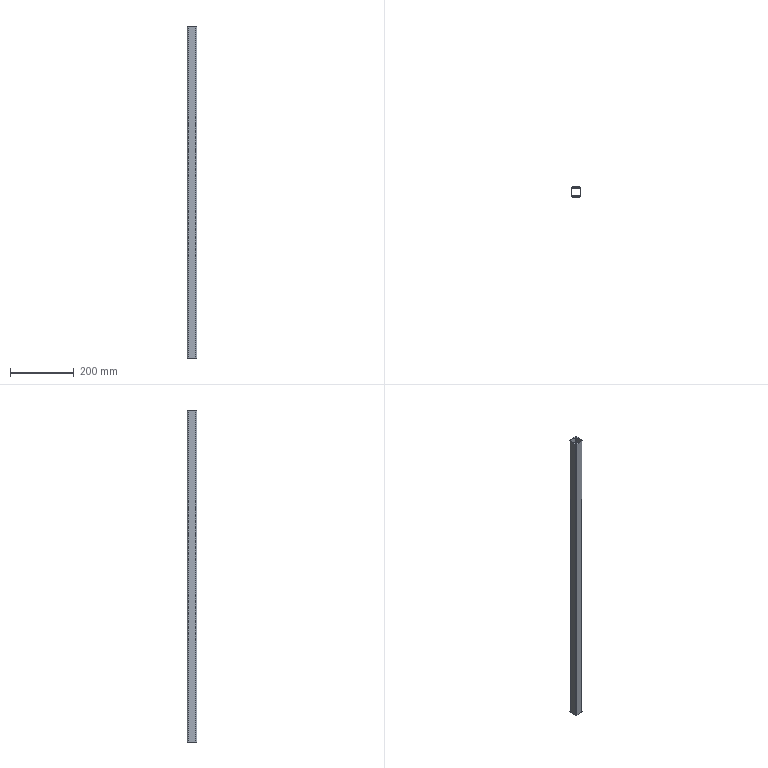Part | SolidWorks | features Attribute 1, ExtruThin 1 | 1 solid | 18 faces | box 30 x 30 x 1038 mm | volume 221734 mm3 | plane 10 | cylinder 8 | commonest cylinder face diameters 4 x4 8 x4
STEP:
#1=CARTESIAN_POINT('',(15.,11.,518.8));
#2=VERTEX_POINT('',#1);
#3=CARTESIAN_POINT('',(11.,15.,518.8));
#4=VERTEX_POINT('',#3);
#5=CARTESIAN_POINT('',(11.,11.,518.8));
#6=DIRECTION('',(0.,0.,1.));
#7=DIRECTION('',(1.,0.,0.));
#8=AXIS2_PLACEMENT_3D('',#5,#6,#7);
#9=CIRCLE('',#8,4.);
#10=EDGE_CURVE('',#2,#4,#9,.T.);
#11=ORIENTED_EDGE('',*,*,#10,.T.);
#12=CARTESIAN_POINT('',(-11.,15.,518.8));
#13=VERTEX_POINT('',#12);
#14=CARTESIAN_POINT('',(11.,15.,518.8));
#15=DIRECTION('',(-1.,0.,0.));
#16=VECTOR('',#15,1000.);
#17=LINE('',#14,#16);
#18=EDGE_CURVE('',#4,#13,#17,.T.);
#19=ORIENTED_EDGE('',*,*,#18,.T.);
#20=CARTESIAN_POINT('',(-15.,11.,518.8));
#21=VERTEX_POINT('',#20);
#22=CARTESIAN_POINT('',(-11.,11.,518.8));
#23=DIRECTION('',(0.,0.,1.));
#24=DIRECTION('',(1.,0.,0.));
#25=AXIS2_PLACEMENT_3D('',#22,#23,#24);
#26=CIRCLE('',#25,4.);
#27=EDGE_CURVE('',#13,#21,#26,.T.);
#28=ORIENTED_EDGE('',*,*,#27,.T.);
#29=CARTESIAN_POINT('',(-15.,-11.,518.8));
#30=VERTEX_POINT('',#29);
#31=CARTESIAN_POINT('',(-15.,-11.,518.8));
#32=DIRECTION('',(0.,1.,0.));
#33=VECTOR('',#32,1000.);
#34=LINE('',#31,#33);
#35=EDGE_CURVE('',#30,#21,#34,.T.);
#36=ORIENTED_EDGE('',*,*,#35,.F.);
#37=CARTESIAN_POINT('',(-11.,-15.,518.8));
#38=VERTEX_POINT('',#37);
#39=CARTESIAN_POINT('',(-11.,-11.,518.8));
#40=DIRECTION('',(0.,0.,1.));
#41=DIRECTION('',(1.,0.,0.));
#42=AXIS2_PLACEMENT_3D('',#39,#40,#41);
#43=CIRCLE('',#42,4.);
#44=EDGE_CURVE('',#30,#38,#43,.T.);
#45=ORIENTED_EDGE('',*,*,#44,.T.);
#46=CARTESIAN_POINT('',(11.,-15.,518.8));
#47=VERTEX_POINT('',#46);
#48=CARTESIAN_POINT('',(-11.,-15.,518.8));
#49=DIRECTION('',(1.,0.,0.));
#50=VECTOR('',#49,1000.);
#51=LINE('',#48,#50);
#52=EDGE_CURVE('',#38,#47,#51,.T.);
#53=ORIENTED_EDGE('',*,*,#52,.T.);
#54=CARTESIAN_POINT('',(15.,-11.,518.8));
#55=VERTEX_POINT('',#54);
#56=CARTESIAN_POINT('',(11.,-11.,518.8));
#57=DIRECTION('',(0.,0.,1.));
#58=DIRECTION('',(1.,0.,0.));
#59=AXIS2_PLACEMENT_3D('',#56,#57,#58);
#60=CIRCLE('',#59,4.);
#61=EDGE_CURVE('',#47,#55,#60,.T.);
#62=ORIENTED_EDGE('',*,*,#61,.T.);
#63=CARTESIAN_POINT('',(15.,11.,518.8));
#64=DIRECTION('',(0.,-1.,0.));
#65=VECTOR('',#64,1000.);
#66=LINE('',#63,#65);
#67=EDGE_CURVE('',#2,#55,#66,.T.);
#68=ORIENTED_EDGE('',*,*,#67,.F.);
#69=EDGE_LOOP('',(#11,#19,#28,#36,#45,#53,#62,#68));
#70=FACE_OUTER_BOUND('',#69,.T.);
#71=CARTESIAN_POINT('',(11.,13.,518.8));
#72=VERTEX_POINT('',#71);
#73=CARTESIAN_POINT('',(-11.,13.,518.8));
#74=VERTEX_POINT('',#73);
#75=CARTESIAN_POINT('',(11.,13.,518.8));
#76=DIRECTION('',(-1.,0.,0.));
#77=VECTOR('',#76,1000.);
#78=LINE('',#75,#77);
#79=EDGE_CURVE('',#72,#74,#78,.T.);
#80=ORIENTED_EDGE('',*,*,#79,.F.);
#81=CARTESIAN_POINT('',(13.,11.,518.8));
#82=VERTEX_POINT('',#81);
#83=CARTESIAN_POINT('',(11.,11.,518.8));
#84=DIRECTION('',(0.,0.,1.));
#85=DIRECTION('',(1.,0.,0.));
#86=AXIS2_PLACEMENT_3D('',#83,#84,#85);
#87=CIRCLE('',#86,2.);
#88=EDGE_CURVE('',#82,#72,#87,.T.);
#89=ORIENTED_EDGE('',*,*,#88,.F.);
#90=CARTESIAN_POINT('',(13.,-11.,518.8));
#91=VERTEX_POINT('',#90);
#92=CARTESIAN_POINT('',(13.,11.,518.8));
#93=DIRECTION('',(0.,-1.,0.));
#94=VECTOR('',#93,1000.);
#95=LINE('',#92,#94);
#96=EDGE_CURVE('',#82,#91,#95,.T.);
#97=ORIENTED_EDGE('',*,*,#96,.T.);
#98=CARTESIAN_POINT('',(11.,-13.,518.8));
#99=VERTEX_POINT('',#98);
#100=CARTESIAN_POINT('',(11.,-11.,518.8));
#101=DIRECTION('',(0.,0.,1.));
#102=DIRECTION('',(1.,0.,0.));
#103=AXIS2_PLACEMENT_3D('',#100,#101,#102);
#104=CIRCLE('',#103,2.);
#105=EDGE_CURVE('',#99,#91,#104,.T.);
#106=ORIENTED_EDGE('',*,*,#105,.F.);
#107=CARTESIAN_POINT('',(-11.,-13.,518.8));
#108=VERTEX_POINT('',#107);
#109=CARTESIAN_POINT('',(-11.,-13.,518.8));
#110=DIRECTION('',(1.,0.,0.));
#111=VECTOR('',#110,1000.);
#112=LINE('',#109,#111);
#113=EDGE_CURVE('',#108,#99,#112,.T.);
#114=ORIENTED_EDGE('',*,*,#113,.F.);
#115=CARTESIAN_POINT('',(-13.,-11.,518.8));
#116=VERTEX_POINT('',#115);
#117=CARTESIAN_POINT('',(-11.,-11.,518.8));
#118=DIRECTION('',(0.,0.,1.));
#119=DIRECTION('',(1.,0.,0.));
#120=AXIS2_PLACEMENT_3D('',#117,#118,#119);
#121=CIRCLE('',#120,2.);
#122=EDGE_CURVE('',#116,#108,#121,.T.);
#123=ORIENTED_EDGE('',*,*,#122,.F.);
#124=CARTESIAN_POINT('',(-13.,11.,518.8));
#125=VERTEX_POINT('',#124);
#126=CARTESIAN_POINT('',(-13.,-11.,518.8));
#127=DIRECTION('',(0.,1.,0.));
#128=VECTOR('',#127,1000.);
#129=LINE('',#126,#128);
#130=EDGE_CURVE('',#116,#125,#129,.T.);
#131=ORIENTED_EDGE('',*,*,#130,.T.);
#132=CARTESIAN_POINT('',(-11.,11.,518.8));
#133=DIRECTION('',(0.,0.,1.));
#134=DIRECTION('',(1.,0.,0.));
#135=AXIS2_PLACEMENT_3D('',#132,#133,#134);
#136=CIRCLE('',#135,2.);
#137=EDGE_CURVE('',#74,#125,#136,.T.);
#138=ORIENTED_EDGE('',*,*,#137,.F.);
#139=EDGE_LOOP('',(#80,#89,#97,#106,#114,#123,#131,#138));
#140=FACE_BOUND('',#139,.T.);
#141=CARTESIAN_POINT('',(11.,11.,518.8));
#142=DIRECTION('',(0.,0.,1.));
#143=DIRECTION('',(1.,0.,0.));
#144=AXIS2_PLACEMENT_3D('',#141,#142,#143);
#145=PLANE('',#144);
#146=ADVANCED_FACE('',(#70,#140),#145,.T.);
#147=CARTESIAN_POINT('',(15.,11.,-518.8));
#148=VERTEX_POINT('',#147);
#149=CARTESIAN_POINT('',(11.,15.,-518.8));
#150=VERTEX_POINT('',#149);
#151=CARTESIAN_POINT('',(11.,11.,-518.8));
#152=DIRECTION('',(0.,0.,1.));
#153=DIRECTION('',(1.,0.,0.));
#154=AXIS2_PLACEMENT_3D('',#151,#152,#153);
#155=CIRCLE('',#154,4.);
#156=EDGE_CURVE('',#148,#150,#155,.T.);
#157=ORIENTED_EDGE('',*,*,#156,.F.);
#158=CARTESIAN_POINT('',(15.,-11.,-518.8));
#159=VERTEX_POINT('',#158);
#160=CARTESIAN_POINT('',(15.,11.,-518.8));
#161=DIRECTION('',(0.,-1.,0.));
#162=VECTOR('',#161,1000.);
#163=LINE('',#160,#162);
#164=EDGE_CURVE('',#148,#159,#163,.T.);
#165=ORIENTED_EDGE('',*,*,#164,.T.);
#166=CARTESIAN_POINT('',(11.,-15.,-518.8));
#167=VERTEX_POINT('',#166);
#168=CARTESIAN_POINT('',(11.,-11.,-518.8));
#169=DIRECTION('',(0.,0.,1.));
#170=DIRECTION('',(1.,0.,0.));
#171=AXIS2_PLACEMENT_3D('',#168,#169,#170);
#172=CIRCLE('',#171,4.);
#173=EDGE_CURVE('',#167,#159,#172,.T.);
#174=ORIENTED_EDGE('',*,*,#173,.F.);
#175=CARTESIAN_POINT('',(-11.,-15.,-518.8));
#176=VERTEX_POINT('',#175);
#177=CARTESIAN_POINT('',(-11.,-15.,-518.8));
#178=DIRECTION('',(1.,0.,0.));
#179=VECTOR('',#178,1000.);
#180=LINE('',#177,#179);
#181=EDGE_CURVE('',#176,#167,#180,.T.);
#182=ORIENTED_EDGE('',*,*,#181,.F.);
#183=CARTESIAN_POINT('',(-15.,-11.,-518.8));
#184=VERTEX_POINT('',#183);
#185=CARTESIAN_POINT('',(-11.,-11.,-518.8));
#186=DIRECTION('',(0.,0.,1.));
#187=DIRECTION('',(1.,0.,0.));
#188=AXIS2_PLACEMENT_3D('',#185,#186,#187);
#189=CIRCLE('',#188,4.);
#190=EDGE_CURVE('',#184,#176,#189,.T.);
#191=ORIENTED_EDGE('',*,*,#190,.F.);
#192=CARTESIAN_POINT('',(-15.,11.,-518.8));
#193=VERTEX_POINT('',#192);
#194=CARTESIAN_POINT('',(-15.,-11.,-518.8));
#195=DIRECTION('',(0.,1.,0.));
#196=VECTOR('',#195,1000.);
#197=LINE('',#194,#196);
#198=EDGE_CURVE('',#184,#193,#197,.T.);
#199=ORIENTED_EDGE('',*,*,#198,.T.);
#200=CARTESIAN_POINT('',(-11.,15.,-518.8));
#201=VERTEX_POINT('',#200);
#202=CARTESIAN_POINT('',(-11.,11.,-518.8));
#203=DIRECTION('',(0.,0.,1.));
#204=DIRECTION('',(1.,0.,0.));
#205=AXIS2_PLACEMENT_3D('',#202,#203,#204);
#206=CIRCLE('',#205,4.);
#207=EDGE_CURVE('',#201,#193,#206,.T.);
#208=ORIENTED_EDGE('',*,*,#207,.F.);
#209=CARTESIAN_POINT('',(11.,15.,-518.8));
#210=DIRECTION('',(-1.,0.,0.));
#211=VECTOR('',#210,1000.);
#212=LINE('',#209,#211);
#213=EDGE_CURVE('',#150,#201,#212,.T.);
#214=ORIENTED_EDGE('',*,*,#213,.F.);
#215=EDGE_LOOP('',(#157,#165,#174,#182,#191,#199,#208,#214));
#216=FACE_OUTER_BOUND('',#215,.T.);
#217=CARTESIAN_POINT('',(13.,11.,-518.8));
#218=VERTEX_POINT('',#217);
#219=CARTESIAN_POINT('',(11.,13.,-518.8));
#220=VERTEX_POINT('',#219);
#221=CARTESIAN_POINT('',(11.,11.,-518.8));
#222=DIRECTION('',(0.,0.,1.));
#223=DIRECTION('',(1.,0.,0.));
#224=AXIS2_PLACEMENT_3D('',#221,#222,#223);
#225=CIRCLE('',#224,2.);
#226=EDGE_CURVE('',#218,#220,#225,.T.);
#227=ORIENTED_EDGE('',*,*,#226,.T.);
#228=CARTESIAN_POINT('',(-11.,13.,-518.8));
#229=VERTEX_POINT('',#228);
#230=CARTESIAN_POINT('',(11.,13.,-518.8));
#231=DIRECTION('',(-1.,0.,0.));
#232=VECTOR('',#231,1000.);
#233=LINE('',#230,#232);
#234=EDGE_CURVE('',#220,#229,#233,.T.);
#235=ORIENTED_EDGE('',*,*,#234,.T.);
#236=CARTESIAN_POINT('',(-13.,11.,-518.8));
#237=VERTEX_POINT('',#236);
#238=CARTESIAN_POINT('',(-11.,11.,-518.8));
#239=DIRECTION('',(0.,0.,1.));
#240=DIRECTION('',(1.,0.,0.));
#241=AXIS2_PLACEMENT_3D('',#238,#239,#240);
#242=CIRCLE('',#241,2.);
#243=EDGE_CURVE('',#229,#237,#242,.T.);
#244=ORIENTED_EDGE('',*,*,#243,.T.);
#245=CARTESIAN_POINT('',(-13.,-11.,-518.8));
#246=VERTEX_POINT('',#245);
#247=CARTESIAN_POINT('',(-13.,-11.,-518.8));
#248=DIRECTION('',(0.,1.,0.));
#249=VECTOR('',#248,1000.);
#250=LINE('',#247,#249);
#251=EDGE_CURVE('',#246,#237,#250,.T.);
#252=ORIENTED_EDGE('',*,*,#251,.F.);
#253=CARTESIAN_POINT('',(-11.,-13.,-518.8));
#254=VERTEX_POINT('',#253);
#255=CARTESIAN_POINT('',(-11.,-11.,-518.8));
#256=DIRECTION('',(0.,0.,1.));
#257=DIRECTION('',(1.,0.,0.));
#258=AXIS2_PLACEMENT_3D('',#255,#256,#257);
#259=CIRCLE('',#258,2.);
#260=EDGE_CURVE('',#246,#254,#259,.T.);
#261=ORIENTED_EDGE('',*,*,#260,.T.);
#262=CARTESIAN_POINT('',(11.,-13.,-518.8));
#263=VERTEX_POINT('',#262);
#264=CARTESIAN_POINT('',(-11.,-13.,-518.8));
#265=DIRECTION('',(1.,0.,0.));
#266=VECTOR('',#265,1000.);
#267=LINE('',#264,#266);
#268=EDGE_CURVE('',#254,#263,#267,.T.);
#269=ORIENTED_EDGE('',*,*,#268,.T.);
#270=CARTESIAN_POINT('',(13.,-11.,-518.8));
#271=VERTEX_POINT('',#270);
#272=CARTESIAN_POINT('',(11.,-11.,-518.8));
#273=DIRECTION('',(0.,0.,1.));
#274=DIRECTION('',(1.,0.,0.));
#275=AXIS2_PLACEMENT_3D('',#272,#273,#274);
#276=CIRCLE('',#275,2.);
#277=EDGE_CURVE('',#263,#271,#276,.T.);
#278=ORIENTED_EDGE('',*,*,#277,.T.);
#279=CARTESIAN_POINT('',(13.,11.,-518.8));
#280=DIRECTION('',(0.,-1.,0.));
#281=VECTOR('',#280,1000.);
#282=LINE('',#279,#281);
#283=EDGE_CURVE('',#218,#271,#282,.T.);
#284=ORIENTED_EDGE('',*,*,#283,.F.);
#285=EDGE_LOOP('',(#227,#235,#244,#252,#261,#269,#278,#284));
#286=FACE_BOUND('',#285,.T.);
#287=CARTESIAN_POINT('',(11.,11.,-518.8));
#288=DIRECTION('',(0.,0.,1.));
#289=DIRECTION('',(1.,0.,0.));
#290=AXIS2_PLACEMENT_3D('',#287,#288,#289);
#291=PLANE('',#290);
#292=ADVANCED_FACE('',(#216,#286),#291,.F.);
#293=ORIENTED_EDGE('',*,*,#156,.T.);
#294=CARTESIAN_POINT('',(11.,15.,518.8));
#295=DIRECTION('',(0.,0.,-1.));
#296=VECTOR('',#295,1000.);
#297=LINE('',#294,#296);
#298=EDGE_CURVE('',#4,#150,#297,.T.);
#299=ORIENTED_EDGE('',*,*,#298,.F.);
#300=ORIENTED_EDGE('',*,*,#10,.F.);
#301=CARTESIAN_POINT('',(15.,11.,518.8));
#302=DIRECTION('',(0.,0.,-1.));
#303=VECTOR('',#302,1000.);
#304=LINE('',#301,#303);
#305=EDGE_CURVE('',#2,#148,#304,.T.);
#306=ORIENTED_EDGE('',*,*,#305,.T.);
#307=EDGE_LOOP('',(#293,#299,#300,#306));
#308=FACE_OUTER_BOUND('',#307,.T.);
#309=CARTESIAN_POINT('',(11.,11.,518.8));
#310=DIRECTION('',(0.,0.,-1.));
#311=DIRECTION('',(-1.,0.,0.));
#312=AXIS2_PLACEMENT_3D('',#309,#310,#311);
#313=CYLINDRICAL_SURFACE('',#312,4.);
#314=ADVANCED_FACE('',(#308),#313,.T.);
#315=ORIENTED_EDGE('',*,*,#213,.T.);
#316=CARTESIAN_POINT('',(-11.,15.,518.8));
#317=DIRECTION('',(0.,0.,-1.));
#318=VECTOR('',#317,1000.);
#319=LINE('',#316,#318);
#320=EDGE_CURVE('',#13,#201,#319,.T.);
#321=ORIENTED_EDGE('',*,*,#320,.F.);
#322=ORIENTED_EDGE('',*,*,#18,.F.);
#323=ORIENTED_EDGE('',*,*,#298,.T.);
#324=EDGE_LOOP('',(#315,#321,#322,#323));
#325=FACE_OUTER_BOUND('',#324,.T.);
#326=CARTESIAN_POINT('',(11.,15.,518.8));
#327=DIRECTION('',(0.,-1.,0.));
#328=DIRECTION('',(0.,0.,-1.));
#329=AXIS2_PLACEMENT_3D('',#326,#327,#328);
#330=PLANE('',#329);
#331=ADVANCED_FACE('',(#325),#330,.F.);
#332=ORIENTED_EDGE('',*,*,#207,.T.);
#333=CARTESIAN_POINT('',(-15.,11.,518.8));
#334=DIRECTION('',(0.,0.,-1.));
#335=VECTOR('',#334,1000.);
#336=LINE('',#333,#335);
#337=EDGE_CURVE('',#21,#193,#336,.T.);
#338=ORIENTED_EDGE('',*,*,#337,.F.);
#339=ORIENTED_EDGE('',*,*,#27,.F.);
#340=ORIENTED_EDGE('',*,*,#320,.T.);
#341=EDGE_LOOP('',(#332,#338,#339,#340));
#342=FACE_OUTER_BOUND('',#341,.T.);
#343=CARTESIAN_POINT('',(-11.,11.,518.8));
#344=DIRECTION('',(0.,0.,-1.));
#345=DIRECTION('',(-1.,0.,0.));
#346=AXIS2_PLACEMENT_3D('',#343,#344,#345);
#347=CYLINDRICAL_SURFACE('',#346,4.);
#348=ADVANCED_FACE('',(#342),#347,.T.);
#349=ORIENTED_EDGE('',*,*,#198,.F.);
#350=CARTESIAN_POINT('',(-15.,-11.,518.8));
#351=DIRECTION('',(0.,0.,-1.));
#352=VECTOR('',#351,1000.);
#353=LINE('',#350,#352);
#354=EDGE_CURVE('',#30,#184,#353,.T.);
#355=ORIENTED_EDGE('',*,*,#354,.F.);
#356=ORIENTED_EDGE('',*,*,#35,.T.);
#357=ORIENTED_EDGE('',*,*,#337,.T.);
#358=EDGE_LOOP('',(#349,#355,#356,#357));
#359=FACE_OUTER_BOUND('',#358,.T.);
#360=CARTESIAN_POINT('',(-15.,-11.,518.8));
#361=DIRECTION('',(-1.,0.,0.));
#362=DIRECTION('',(0.,0.,1.));
#363=AXIS2_PLACEMENT_3D('',#360,#361,#362);
#364=PLANE('',#363);
#365=ADVANCED_FACE('',(#359),#364,.T.);
#366=ORIENTED_EDGE('',*,*,#190,.T.);
#367=CARTESIAN_POINT('',(-11.,-15.,518.8));
#368=DIRECTION('',(0.,0.,-1.));
#369=VECTOR('',#368,1000.);
#370=LINE('',#367,#369);
#371=EDGE_CURVE('',#38,#176,#370,.T.);
#372=ORIENTED_EDGE('',*,*,#371,.F.);
#373=ORIENTED_EDGE('',*,*,#44,.F.);
#374=ORIENTED_EDGE('',*,*,#354,.T.);
#375=EDGE_LOOP('',(#366,#372,#373,#374));
#376=FACE_OUTER_BOUND('',#375,.T.);
#377=CARTESIAN_POINT('',(-11.,-11.,518.8));
#378=DIRECTION('',(0.,0.,-1.));
#379=DIRECTION('',(-1.,0.,0.));
#380=AXIS2_PLACEMENT_3D('',#377,#378,#379);
#381=CYLINDRICAL_SURFACE('',#380,4.);
#382=ADVANCED_FACE('',(#376),#381,.T.);
#383=ORIENTED_EDGE('',*,*,#181,.T.);
#384=CARTESIAN_POINT('',(11.,-15.,518.8));
#385=DIRECTION('',(0.,0.,-1.));
#386=VECTOR('',#385,1000.);
#387=LINE('',#384,#386);
#388=EDGE_CURVE('',#47,#167,#387,.T.);
#389=ORIENTED_EDGE('',*,*,#388,.F.);
#390=ORIENTED_EDGE('',*,*,#52,.F.);
#391=ORIENTED_EDGE('',*,*,#371,.T.);
#392=EDGE_LOOP('',(#383,#389,#390,#391));
#393=FACE_OUTER_BOUND('',#392,.T.);
#394=CARTESIAN_POINT('',(-11.,-15.,518.8));
#395=DIRECTION('',(0.,1.,0.));
#396=DIRECTION('',(0.,0.,1.));
#397=AXIS2_PLACEMENT_3D('',#394,#395,#396);
#398=PLANE('',#397);
#399=ADVANCED_FACE('',(#393),#398,.F.);
#400=ORIENTED_EDGE('',*,*,#173,.T.);
#401=CARTESIAN_POINT('',(15.,-11.,518.8));
#402=DIRECTION('',(0.,0.,-1.));
#403=VECTOR('',#402,1000.);
#404=LINE('',#401,#403);
#405=EDGE_CURVE('',#55,#159,#404,.T.);
#406=ORIENTED_EDGE('',*,*,#405,.F.);
#407=ORIENTED_EDGE('',*,*,#61,.F.);
#408=ORIENTED_EDGE('',*,*,#388,.T.);
#409=EDGE_LOOP('',(#400,#406,#407,#408));
#410=FACE_OUTER_BOUND('',#409,.T.);
#411=CARTESIAN_POINT('',(11.,-11.,518.8));
#412=DIRECTION('',(0.,0.,-1.));
#413=DIRECTION('',(-1.,0.,0.));
#414=AXIS2_PLACEMENT_3D('',#411,#412,#413);
#415=CYLINDRICAL_SURFACE('',#414,4.);
#416=ADVANCED_FACE('',(#410),#415,.T.);
#417=ORIENTED_EDGE('',*,*,#164,.F.);
#418=ORIENTED_EDGE('',*,*,#305,.F.);
#419=ORIENTED_EDGE('',*,*,#67,.T.);
#420=ORIENTED_EDGE('',*,*,#405,.T.);
#421=EDGE_LOOP('',(#417,#418,#419,#420));
#422=FACE_OUTER_BOUND('',#421,.T.);
#423=CARTESIAN_POINT('',(15.,11.,518.8));
#424=DIRECTION('',(1.,0.,0.));
#425=DIRECTION('',(0.,0.,-1.));
#426=AXIS2_PLACEMENT_3D('',#423,#424,#425);
#427=PLANE('',#426);
#428=ADVANCED_FACE('',(#422),#427,.T.);
#429=ORIENTED_EDGE('',*,*,#226,.F.);
#430=CARTESIAN_POINT('',(13.,11.,518.8));
#431=DIRECTION('',(0.,0.,-1.));
#432=VECTOR('',#431,1000.);
#433=LINE('',#430,#432);
#434=EDGE_CURVE('',#82,#218,#433,.T.);
#435=ORIENTED_EDGE('',*,*,#434,.F.);
#436=ORIENTED_EDGE('',*,*,#88,.T.);
#437=CARTESIAN_POINT('',(11.,13.,518.8));
#438=DIRECTION('',(0.,0.,-1.));
#439=VECTOR('',#438,1000.);
#440=LINE('',#437,#439);
#441=EDGE_CURVE('',#72,#220,#440,.T.);
#442=ORIENTED_EDGE('',*,*,#441,.T.);
#443=EDGE_LOOP('',(#429,#435,#436,#442));
#444=FACE_OUTER_BOUND('',#443,.T.);
#445=CARTESIAN_POINT('',(11.,11.,518.8));
#446=DIRECTION('',(0.,0.,-1.));
#447=DIRECTION('',(-1.,0.,0.));
#448=AXIS2_PLACEMENT_3D('',#445,#446,#447);
#449=CYLINDRICAL_SURFACE('',#448,2.);
#450=ADVANCED_FACE('',(#444),#449,.F.);
#451=ORIENTED_EDGE('',*,*,#234,.F.);
#452=ORIENTED_EDGE('',*,*,#441,.F.);
#453=ORIENTED_EDGE('',*,*,#79,.T.);
#454=CARTESIAN_POINT('',(-11.,13.,518.8));
#455=DIRECTION('',(0.,0.,-1.));
#456=VECTOR('',#455,1000.);
#457=LINE('',#454,#456);
#458=EDGE_CURVE('',#74,#229,#457,.T.);
#459=ORIENTED_EDGE('',*,*,#458,.T.);
#460=EDGE_LOOP('',(#451,#452,#453,#459));
#461=FACE_OUTER_BOUND('',#460,.T.);
#462=CARTESIAN_POINT('',(11.,13.,518.8));
#463=DIRECTION('',(0.,-1.,0.));
#464=DIRECTION('',(0.,0.,-1.));
#465=AXIS2_PLACEMENT_3D('',#462,#463,#464);
#466=PLANE('',#465);
#467=ADVANCED_FACE('',(#461),#466,.T.);
#468=ORIENTED_EDGE('',*,*,#243,.F.);
#469=ORIENTED_EDGE('',*,*,#458,.F.);
#470=ORIENTED_EDGE('',*,*,#137,.T.);
#471=CARTESIAN_POINT('',(-13.,11.,518.8));
#472=DIRECTION('',(0.,0.,-1.));
#473=VECTOR('',#472,1000.);
#474=LINE('',#471,#473);
#475=EDGE_CURVE('',#125,#237,#474,.T.);
#476=ORIENTED_EDGE('',*,*,#475,.T.);
#477=EDGE_LOOP('',(#468,#469,#470,#476));
#478=FACE_OUTER_BOUND('',#477,.T.);
#479=CARTESIAN_POINT('',(-11.,11.,518.8));
#480=DIRECTION('',(0.,0.,-1.));
#481=DIRECTION('',(-1.,0.,0.));
#482=AXIS2_PLACEMENT_3D('',#479,#480,#481);
#483=CYLINDRICAL_SURFACE('',#482,2.);
#484=ADVANCED_FACE('',(#478),#483,.F.);
#485=ORIENTED_EDGE('',*,*,#251,.T.);
#486=ORIENTED_EDGE('',*,*,#475,.F.);
#487=ORIENTED_EDGE('',*,*,#130,.F.);
#488=CARTESIAN_POINT('',(-13.,-11.,518.8));
#489=DIRECTION('',(0.,0.,-1.));
#490=VECTOR('',#489,1000.);
#491=LINE('',#488,#490);
#492=EDGE_CURVE('',#116,#246,#491,.T.);
#493=ORIENTED_EDGE('',*,*,#492,.T.);
#494=EDGE_LOOP('',(#485,#486,#487,#493));
#495=FACE_OUTER_BOUND('',#494,.T.);
#496=CARTESIAN_POINT('',(-13.,-11.,518.8));
#497=DIRECTION('',(-1.,0.,0.));
#498=DIRECTION('',(0.,0.,1.));
#499=AXIS2_PLACEMENT_3D('',#496,#497,#498);
#500=PLANE('',#499);
#501=ADVANCED_FACE('',(#495),#500,.F.);
#502=ORIENTED_EDGE('',*,*,#260,.F.);
#503=ORIENTED_EDGE('',*,*,#492,.F.);
#504=ORIENTED_EDGE('',*,*,#122,.T.);
#505=CARTESIAN_POINT('',(-11.,-13.,518.8));
#506=DIRECTION('',(0.,0.,-1.));
#507=VECTOR('',#506,1000.);
#508=LINE('',#505,#507);
#509=EDGE_CURVE('',#108,#254,#508,.T.);
#510=ORIENTED_EDGE('',*,*,#509,.T.);
#511=EDGE_LOOP('',(#502,#503,#504,#510));
#512=FACE_OUTER_BOUND('',#511,.T.);
#513=CARTESIAN_POINT('',(-11.,-11.,518.8));
#514=DIRECTION('',(0.,0.,-1.));
#515=DIRECTION('',(-1.,0.,0.));
#516=AXIS2_PLACEMENT_3D('',#513,#514,#515);
#517=CYLINDRICAL_SURFACE('',#516,2.);
#518=ADVANCED_FACE('',(#512),#517,.F.);
#519=ORIENTED_EDGE('',*,*,#268,.F.);
#520=ORIENTED_EDGE('',*,*,#509,.F.);
#521=ORIENTED_EDGE('',*,*,#113,.T.);
#522=CARTESIAN_POINT('',(11.,-13.,518.8));
#523=DIRECTION('',(0.,0.,-1.));
#524=VECTOR('',#523,1000.);
#525=LINE('',#522,#524);
#526=EDGE_CURVE('',#99,#263,#525,.T.);
#527=ORIENTED_EDGE('',*,*,#526,.T.);
#528=EDGE_LOOP('',(#519,#520,#521,#527));
#529=FACE_OUTER_BOUND('',#528,.T.);
#530=CARTESIAN_POINT('',(-11.,-13.,518.8));
#531=DIRECTION('',(0.,1.,0.));
#532=DIRECTION('',(0.,0.,1.));
#533=AXIS2_PLACEMENT_3D('',#530,#531,#532);
#534=PLANE('',#533);
#535=ADVANCED_FACE('',(#529),#534,.T.);
#536=ORIENTED_EDGE('',*,*,#277,.F.);
#537=ORIENTED_EDGE('',*,*,#526,.F.);
#538=ORIENTED_EDGE('',*,*,#105,.T.);
#539=CARTESIAN_POINT('',(13.,-11.,518.8));
#540=DIRECTION('',(0.,0.,-1.));
#541=VECTOR('',#540,1000.);
#542=LINE('',#539,#541);
#543=EDGE_CURVE('',#91,#271,#542,.T.);
#544=ORIENTED_EDGE('',*,*,#543,.T.);
#545=EDGE_LOOP('',(#536,#537,#538,#544));
#546=FACE_OUTER_BOUND('',#545,.T.);
#547=CARTESIAN_POINT('',(11.,-11.,518.8));
#548=DIRECTION('',(0.,0.,-1.));
#549=DIRECTION('',(-1.,0.,0.));
#550=AXIS2_PLACEMENT_3D('',#547,#548,#549);
#551=CYLINDRICAL_SURFACE('',#550,2.);
#552=ADVANCED_FACE('',(#546),#551,.F.);
#553=ORIENTED_EDGE('',*,*,#283,.T.);
#554=ORIENTED_EDGE('',*,*,#543,.F.);
#555=ORIENTED_EDGE('',*,*,#96,.F.);
#556=ORIENTED_EDGE('',*,*,#434,.T.);
#557=EDGE_LOOP('',(#553,#554,#555,#556));
#558=FACE_OUTER_BOUND('',#557,.T.);
#559=CARTESIAN_POINT('',(13.,11.,518.8));
#560=DIRECTION('',(1.,0.,0.));
#561=DIRECTION('',(0.,0.,-1.));
#562=AXIS2_PLACEMENT_3D('',#559,#560,#561);
#563=PLANE('',#562);
#564=ADVANCED_FACE('',(#558),#563,.F.);
#565=CLOSED_SHELL('',(#146,#292,#314,#331,#348,#365,#382,#399,#416,#428,#450,#467,#484,#501,#518,#535,#552,#564));
#566=MANIFOLD_SOLID_BREP('',#565);
#567=CARTESIAN_POINT('',(0.,0.,0.));
#568=DIRECTION('',(0.,0.,1.));
#569=DIRECTION('',(1.,0.,0.));
#570=AXIS2_PLACEMENT_3D('',#567,#568,#569);
#571=(LENGTH_UNIT()NAMED_UNIT(*)SI_UNIT(.MILLI.,.METRE.));
#572=UNCERTAINTY_MEASURE_WITH_UNIT(LENGTH_MEASURE(0.00001),#571,'','');
#573=(NAMED_UNIT(*)PLANE_ANGLE_UNIT()SI_UNIT($,.RADIAN.));
#574=(NAMED_UNIT(*)SI_UNIT($,.STERADIAN.)SOLID_ANGLE_UNIT());
#575=(GEOMETRIC_REPRESENTATION_CONTEXT(3)GLOBAL_UNCERTAINTY_ASSIGNED_CONTEXT((#572))GLOBAL_UNIT_ASSIGNED_CONTEXT((#571,#573,#574))REPRESENTATION_CONTEXT('',''));
#576=ADVANCED_BREP_SHAPE_REPRESENTATION('',(#566,#570),#575);